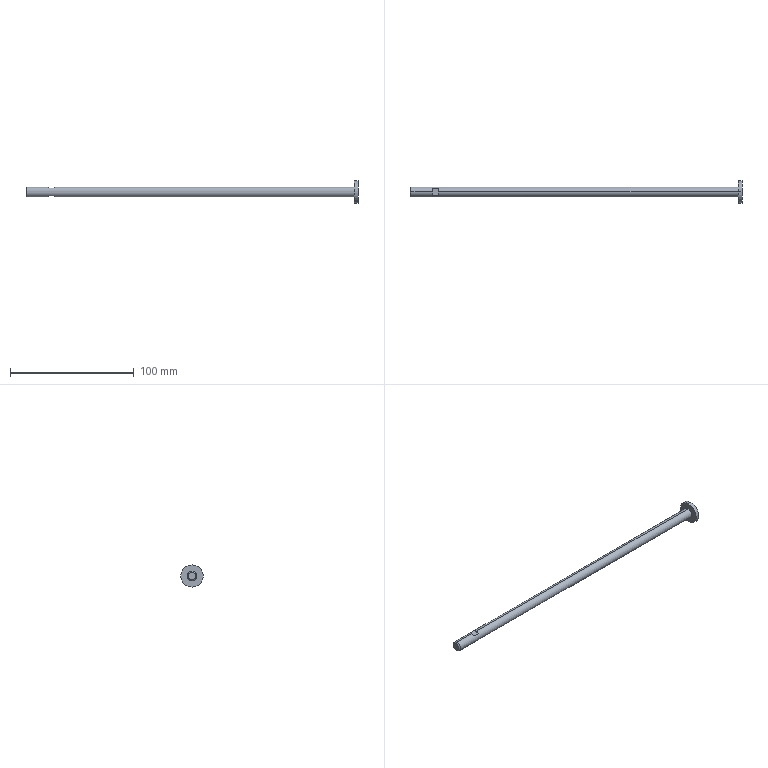Part | 1 solid | 15 faces | box 268 x 18 x 18 mm | volume 14041 mm3 | plane 9 | cylinder 4 | cone 2 | commonest cylinder face diameters 8 x2 18 x2
STEP:
#1=CARTESIAN_POINT('',(265.,0.,-9.));
#2=VERTEX_POINT('',#1);
#3=CARTESIAN_POINT('',(265.,0.,9.));
#4=VERTEX_POINT('',#3);
#5=CARTESIAN_POINT('',(265.,0.,0.));
#6=DIRECTION('',(1.,0.,0.));
#7=DIRECTION('',(0.,0.,-1.));
#8=AXIS2_PLACEMENT_3D('',#5,#6,#7);
#9=CIRCLE('',#8,9.);
#10=EDGE_CURVE('',#2,#4,#9,.T.);
#11=ORIENTED_EDGE('',*,*,#10,.T.);
#12=CARTESIAN_POINT('',(268.,0.,9.));
#13=VERTEX_POINT('',#12);
#14=CARTESIAN_POINT('',(268.,0.,9.));
#15=DIRECTION('',(1.,0.,0.));
#16=VECTOR('',#15,1000.);
#17=LINE('',#14,#16);
#18=EDGE_CURVE('',#4,#13,#17,.T.);
#19=ORIENTED_EDGE('',*,*,#18,.T.);
#20=CARTESIAN_POINT('',(268.,0.,-9.));
#21=VERTEX_POINT('',#20);
#22=CARTESIAN_POINT('',(268.,0.,0.));
#23=DIRECTION('',(1.,0.,0.));
#24=DIRECTION('',(0.,0.,-1.));
#25=AXIS2_PLACEMENT_3D('',#22,#23,#24);
#26=CIRCLE('',#25,9.);
#27=EDGE_CURVE('',#21,#13,#26,.T.);
#28=ORIENTED_EDGE('',*,*,#27,.F.);
#29=CARTESIAN_POINT('',(268.,0.,-9.));
#30=DIRECTION('',(1.,0.,0.));
#31=VECTOR('',#30,1000.);
#32=LINE('',#29,#31);
#33=EDGE_CURVE('',#2,#21,#32,.T.);
#34=ORIENTED_EDGE('',*,*,#33,.F.);
#35=EDGE_LOOP('',(#11,#19,#28,#34));
#36=FACE_OUTER_BOUND('',#35,.T.);
#37=CARTESIAN_POINT('',(268.,0.,0.));
#38=DIRECTION('',(1.,0.,0.));
#39=DIRECTION('',(0.,0.,-1.));
#40=AXIS2_PLACEMENT_3D('',#37,#38,#39);
#41=CYLINDRICAL_SURFACE('',#40,9.);
#42=ADVANCED_FACE('',(#36),#41,.T.);
#43=CARTESIAN_POINT('',(0.767,0.,-4.));
#44=VERTEX_POINT('',#43);
#45=CARTESIAN_POINT('',(0.767,0.,4.));
#46=VERTEX_POINT('',#45);
#47=CARTESIAN_POINT('',(0.767,0.,0.));
#48=DIRECTION('',(1.,0.,0.));
#49=DIRECTION('',(0.,0.,-1.));
#50=AXIS2_PLACEMENT_3D('',#47,#48,#49);
#51=CIRCLE('',#50,4.);
#52=EDGE_CURVE('',#44,#46,#51,.T.);
#53=ORIENTED_EDGE('',*,*,#52,.T.);
#54=CARTESIAN_POINT('',(18.,0.,4.));
#55=VERTEX_POINT('',#54);
#56=CARTESIAN_POINT('',(268.,0.,4.));
#57=DIRECTION('',(1.,0.,0.));
#58=VECTOR('',#57,1000.);
#59=LINE('',#56,#58);
#60=EDGE_CURVE('',#46,#55,#59,.T.);
#61=ORIENTED_EDGE('',*,*,#60,.T.);
#62=CARTESIAN_POINT('',(18.,2.646,3.));
#63=VERTEX_POINT('',#62);
#64=CARTESIAN_POINT('',(18.,0.,0.));
#65=DIRECTION('',(1.,0.,0.));
#66=DIRECTION('',(0.,0.,-1.));
#67=AXIS2_PLACEMENT_3D('',#64,#65,#66);
#68=CIRCLE('',#67,4.);
#69=EDGE_CURVE('',#63,#55,#68,.T.);
#70=ORIENTED_EDGE('',*,*,#69,.F.);
#71=CARTESIAN_POINT('',(23.,2.646,3.));
#72=VERTEX_POINT('',#71);
#73=CARTESIAN_POINT('',(268.,2.646,3.));
#74=DIRECTION('',(1.,0.,0.));
#75=VECTOR('',#74,1000.);
#76=LINE('',#73,#75);
#77=EDGE_CURVE('',#63,#72,#76,.T.);
#78=ORIENTED_EDGE('',*,*,#77,.T.);
#79=CARTESIAN_POINT('',(23.,0.,4.));
#80=VERTEX_POINT('',#79);
#81=CARTESIAN_POINT('',(23.,0.,0.));
#82=DIRECTION('',(1.,0.,0.));
#83=DIRECTION('',(0.,0.,-1.));
#84=AXIS2_PLACEMENT_3D('',#81,#82,#83);
#85=CIRCLE('',#84,4.);
#86=EDGE_CURVE('',#72,#80,#85,.T.);
#87=ORIENTED_EDGE('',*,*,#86,.T.);
#88=CARTESIAN_POINT('',(265.,0.,4.));
#89=VERTEX_POINT('',#88);
#90=CARTESIAN_POINT('',(268.,0.,4.));
#91=DIRECTION('',(1.,0.,0.));
#92=VECTOR('',#91,1000.);
#93=LINE('',#90,#92);
#94=EDGE_CURVE('',#80,#89,#93,.T.);
#95=ORIENTED_EDGE('',*,*,#94,.T.);
#96=CARTESIAN_POINT('',(265.,0.,-4.));
#97=VERTEX_POINT('',#96);
#98=CARTESIAN_POINT('',(265.,0.,0.));
#99=DIRECTION('',(1.,0.,0.));
#100=DIRECTION('',(0.,0.,-1.));
#101=AXIS2_PLACEMENT_3D('',#98,#99,#100);
#102=CIRCLE('',#101,4.);
#103=EDGE_CURVE('',#97,#89,#102,.T.);
#104=ORIENTED_EDGE('',*,*,#103,.F.);
#105=CARTESIAN_POINT('',(23.,0.,-4.));
#106=VERTEX_POINT('',#105);
#107=CARTESIAN_POINT('',(268.,0.,-4.));
#108=DIRECTION('',(1.,0.,0.));
#109=VECTOR('',#108,1000.);
#110=LINE('',#107,#109);
#111=EDGE_CURVE('',#106,#97,#110,.T.);
#112=ORIENTED_EDGE('',*,*,#111,.F.);
#113=CARTESIAN_POINT('',(23.,2.646,-3.));
#114=VERTEX_POINT('',#113);
#115=CARTESIAN_POINT('',(23.,0.,0.));
#116=DIRECTION('',(1.,0.,0.));
#117=DIRECTION('',(0.,0.,-1.));
#118=AXIS2_PLACEMENT_3D('',#115,#116,#117);
#119=CIRCLE('',#118,4.);
#120=EDGE_CURVE('',#106,#114,#119,.T.);
#121=ORIENTED_EDGE('',*,*,#120,.T.);
#122=CARTESIAN_POINT('',(18.,2.646,-3.));
#123=VERTEX_POINT('',#122);
#124=CARTESIAN_POINT('',(268.,2.646,-3.));
#125=DIRECTION('',(-1.,0.,0.));
#126=VECTOR('',#125,1000.);
#127=LINE('',#124,#126);
#128=EDGE_CURVE('',#114,#123,#127,.T.);
#129=ORIENTED_EDGE('',*,*,#128,.T.);
#130=CARTESIAN_POINT('',(18.,0.,-4.));
#131=VERTEX_POINT('',#130);
#132=CARTESIAN_POINT('',(18.,0.,0.));
#133=DIRECTION('',(1.,0.,0.));
#134=DIRECTION('',(0.,0.,-1.));
#135=AXIS2_PLACEMENT_3D('',#132,#133,#134);
#136=CIRCLE('',#135,4.);
#137=EDGE_CURVE('',#131,#123,#136,.T.);
#138=ORIENTED_EDGE('',*,*,#137,.F.);
#139=CARTESIAN_POINT('',(268.,0.,-4.));
#140=DIRECTION('',(1.,0.,0.));
#141=VECTOR('',#140,1000.);
#142=LINE('',#139,#141);
#143=EDGE_CURVE('',#44,#131,#142,.T.);
#144=ORIENTED_EDGE('',*,*,#143,.F.);
#145=EDGE_LOOP('',(#53,#61,#70,#78,#87,#95,#104,#112,#121,#129,#138,#144));
#146=FACE_OUTER_BOUND('',#145,.T.);
#147=CARTESIAN_POINT('',(268.,0.,0.));
#148=DIRECTION('',(1.,0.,0.));
#149=DIRECTION('',(0.,0.,-1.));
#150=AXIS2_PLACEMENT_3D('',#147,#148,#149);
#151=CYLINDRICAL_SURFACE('',#150,4.);
#152=ADVANCED_FACE('',(#146),#151,.T.);
#153=CARTESIAN_POINT('',(0.,0.,-3.233));
#154=VERTEX_POINT('',#153);
#155=CARTESIAN_POINT('',(0.,0.,3.233));
#156=VERTEX_POINT('',#155);
#157=CARTESIAN_POINT('',(0.,0.,0.));
#158=DIRECTION('',(1.,0.,0.));
#159=DIRECTION('',(0.,0.,-1.));
#160=AXIS2_PLACEMENT_3D('',#157,#158,#159);
#161=CIRCLE('',#160,3.233);
#162=EDGE_CURVE('',#154,#156,#161,.T.);
#163=ORIENTED_EDGE('',*,*,#162,.T.);
#164=CARTESIAN_POINT('',(0.,0.,3.233));
#165=DIRECTION('',(0.7071,0.,0.7071));
#166=VECTOR('',#165,1000.);
#167=LINE('',#164,#166);
#168=EDGE_CURVE('',#156,#46,#167,.T.);
#169=ORIENTED_EDGE('',*,*,#168,.T.);
#170=ORIENTED_EDGE('',*,*,#52,.F.);
#171=CARTESIAN_POINT('',(0.,0.,-3.233));
#172=DIRECTION('',(0.7071,0.,-0.7071));
#173=VECTOR('',#172,1000.);
#174=LINE('',#171,#173);
#175=EDGE_CURVE('',#154,#44,#174,.T.);
#176=ORIENTED_EDGE('',*,*,#175,.F.);
#177=EDGE_LOOP('',(#163,#169,#170,#176));
#178=FACE_OUTER_BOUND('',#177,.T.);
#179=CARTESIAN_POINT('',(0.,0.,0.));
#180=DIRECTION('',(1.,0.,0.));
#181=DIRECTION('',(0.,0.,-1.));
#182=AXIS2_PLACEMENT_3D('',#179,#180,#181);
#183=CONICAL_SURFACE('',#182,3.233,0.7854);
#184=ADVANCED_FACE('',(#178),#183,.T.);
#185=ORIENTED_EDGE('',*,*,#162,.F.);
#186=CARTESIAN_POINT('',(0.,0.,0.));
#187=DIRECTION('',(1.,0.,0.));
#188=DIRECTION('',(0.,0.,-1.));
#189=AXIS2_PLACEMENT_3D('',#186,#187,#188);
#190=CIRCLE('',#189,3.233);
#191=EDGE_CURVE('',#156,#154,#190,.T.);
#192=ORIENTED_EDGE('',*,*,#191,.F.);
#193=EDGE_LOOP('',(#185,#192));
#194=FACE_OUTER_BOUND('',#193,.T.);
#195=CARTESIAN_POINT('',(0.,0.,0.));
#196=DIRECTION('',(1.,0.,0.));
#197=DIRECTION('',(0.,1.,0.));
#198=AXIS2_PLACEMENT_3D('',#195,#196,#197);
#199=PLANE('',#198);
#200=ADVANCED_FACE('',(#194),#199,.F.);
#201=ORIENTED_EDGE('',*,*,#168,.F.);
#202=ORIENTED_EDGE('',*,*,#191,.T.);
#203=ORIENTED_EDGE('',*,*,#175,.T.);
#204=CARTESIAN_POINT('',(0.767,0.,0.));
#205=DIRECTION('',(1.,0.,0.));
#206=DIRECTION('',(0.,0.,-1.));
#207=AXIS2_PLACEMENT_3D('',#204,#205,#206);
#208=CIRCLE('',#207,4.);
#209=EDGE_CURVE('',#46,#44,#208,.T.);
#210=ORIENTED_EDGE('',*,*,#209,.F.);
#211=EDGE_LOOP('',(#201,#202,#203,#210));
#212=FACE_OUTER_BOUND('',#211,.T.);
#213=CARTESIAN_POINT('',(0.,0.,0.));
#214=DIRECTION('',(1.,0.,0.));
#215=DIRECTION('',(0.,0.,-1.));
#216=AXIS2_PLACEMENT_3D('',#213,#214,#215);
#217=CONICAL_SURFACE('',#216,3.233,0.7854);
#218=ADVANCED_FACE('',(#212),#217,.T.);
#219=ORIENTED_EDGE('',*,*,#60,.F.);
#220=ORIENTED_EDGE('',*,*,#209,.T.);
#221=ORIENTED_EDGE('',*,*,#143,.T.);
#222=CARTESIAN_POINT('',(18.,-2.646,-3.));
#223=VERTEX_POINT('',#222);
#224=CARTESIAN_POINT('',(18.,0.,0.));
#225=DIRECTION('',(1.,0.,0.));
#226=DIRECTION('',(0.,0.,-1.));
#227=AXIS2_PLACEMENT_3D('',#224,#225,#226);
#228=CIRCLE('',#227,4.);
#229=EDGE_CURVE('',#223,#131,#228,.T.);
#230=ORIENTED_EDGE('',*,*,#229,.F.);
#231=CARTESIAN_POINT('',(23.,-2.646,-3.));
#232=VERTEX_POINT('',#231);
#233=CARTESIAN_POINT('',(268.,-2.646,-3.));
#234=DIRECTION('',(1.,0.,0.));
#235=VECTOR('',#234,1000.);
#236=LINE('',#233,#235);
#237=EDGE_CURVE('',#223,#232,#236,.T.);
#238=ORIENTED_EDGE('',*,*,#237,.T.);
#239=CARTESIAN_POINT('',(23.,0.,0.));
#240=DIRECTION('',(1.,0.,0.));
#241=DIRECTION('',(0.,0.,-1.));
#242=AXIS2_PLACEMENT_3D('',#239,#240,#241);
#243=CIRCLE('',#242,4.);
#244=EDGE_CURVE('',#232,#106,#243,.T.);
#245=ORIENTED_EDGE('',*,*,#244,.T.);
#246=ORIENTED_EDGE('',*,*,#111,.T.);
#247=CARTESIAN_POINT('',(265.,0.,0.));
#248=DIRECTION('',(1.,0.,0.));
#249=DIRECTION('',(0.,0.,-1.));
#250=AXIS2_PLACEMENT_3D('',#247,#248,#249);
#251=CIRCLE('',#250,4.);
#252=EDGE_CURVE('',#89,#97,#251,.T.);
#253=ORIENTED_EDGE('',*,*,#252,.F.);
#254=ORIENTED_EDGE('',*,*,#94,.F.);
#255=CARTESIAN_POINT('',(23.,-2.646,3.));
#256=VERTEX_POINT('',#255);
#257=CARTESIAN_POINT('',(23.,0.,0.));
#258=DIRECTION('',(1.,0.,0.));
#259=DIRECTION('',(0.,0.,-1.));
#260=AXIS2_PLACEMENT_3D('',#257,#258,#259);
#261=CIRCLE('',#260,4.);
#262=EDGE_CURVE('',#80,#256,#261,.T.);
#263=ORIENTED_EDGE('',*,*,#262,.T.);
#264=CARTESIAN_POINT('',(18.,-2.646,3.));
#265=VERTEX_POINT('',#264);
#266=CARTESIAN_POINT('',(268.,-2.646,3.));
#267=DIRECTION('',(-1.,0.,0.));
#268=VECTOR('',#267,1000.);
#269=LINE('',#266,#268);
#270=EDGE_CURVE('',#256,#265,#269,.T.);
#271=ORIENTED_EDGE('',*,*,#270,.T.);
#272=CARTESIAN_POINT('',(18.,0.,0.));
#273=DIRECTION('',(1.,0.,0.));
#274=DIRECTION('',(0.,0.,-1.));
#275=AXIS2_PLACEMENT_3D('',#272,#273,#274);
#276=CIRCLE('',#275,4.);
#277=EDGE_CURVE('',#55,#265,#276,.T.);
#278=ORIENTED_EDGE('',*,*,#277,.F.);
#279=EDGE_LOOP('',(#219,#220,#221,#230,#238,#245,#246,#253,#254,#263,#271,#278));
#280=FACE_OUTER_BOUND('',#279,.T.);
#281=CARTESIAN_POINT('',(268.,0.,0.));
#282=DIRECTION('',(1.,0.,0.));
#283=DIRECTION('',(0.,0.,-1.));
#284=AXIS2_PLACEMENT_3D('',#281,#282,#283);
#285=CYLINDRICAL_SURFACE('',#284,4.);
#286=ADVANCED_FACE('',(#280),#285,.T.);
#287=ORIENTED_EDGE('',*,*,#10,.F.);
#288=CARTESIAN_POINT('',(265.,0.,0.));
#289=DIRECTION('',(1.,0.,0.));
#290=DIRECTION('',(0.,0.,-1.));
#291=AXIS2_PLACEMENT_3D('',#288,#289,#290);
#292=CIRCLE('',#291,9.);
#293=EDGE_CURVE('',#4,#2,#292,.T.);
#294=ORIENTED_EDGE('',*,*,#293,.F.);
#295=EDGE_LOOP('',(#287,#294));
#296=FACE_OUTER_BOUND('',#295,.T.);
#297=ORIENTED_EDGE('',*,*,#103,.T.);
#298=ORIENTED_EDGE('',*,*,#252,.T.);
#299=EDGE_LOOP('',(#297,#298));
#300=FACE_BOUND('',#299,.T.);
#301=CARTESIAN_POINT('',(265.,4.,0.));
#302=DIRECTION('',(1.,0.,0.));
#303=DIRECTION('',(0.,1.,0.));
#304=AXIS2_PLACEMENT_3D('',#301,#302,#303);
#305=PLANE('',#304);
#306=ADVANCED_FACE('',(#296,#300),#305,.F.);
#307=ORIENTED_EDGE('',*,*,#18,.F.);
#308=ORIENTED_EDGE('',*,*,#293,.T.);
#309=ORIENTED_EDGE('',*,*,#33,.T.);
#310=CARTESIAN_POINT('',(268.,0.,0.));
#311=DIRECTION('',(1.,0.,0.));
#312=DIRECTION('',(0.,0.,-1.));
#313=AXIS2_PLACEMENT_3D('',#310,#311,#312);
#314=CIRCLE('',#313,9.);
#315=EDGE_CURVE('',#13,#21,#314,.T.);
#316=ORIENTED_EDGE('',*,*,#315,.F.);
#317=EDGE_LOOP('',(#307,#308,#309,#316));
#318=FACE_OUTER_BOUND('',#317,.T.);
#319=CARTESIAN_POINT('',(268.,0.,0.));
#320=DIRECTION('',(1.,0.,0.));
#321=DIRECTION('',(0.,0.,-1.));
#322=AXIS2_PLACEMENT_3D('',#319,#320,#321);
#323=CYLINDRICAL_SURFACE('',#322,9.);
#324=ADVANCED_FACE('',(#318),#323,.T.);
#325=ORIENTED_EDGE('',*,*,#27,.T.);
#326=ORIENTED_EDGE('',*,*,#315,.T.);
#327=EDGE_LOOP('',(#325,#326));
#328=FACE_OUTER_BOUND('',#327,.T.);
#329=CARTESIAN_POINT('',(268.,9.,0.));
#330=DIRECTION('',(-1.,0.,0.));
#331=DIRECTION('',(0.,0.,1.));
#332=AXIS2_PLACEMENT_3D('',#329,#330,#331);
#333=PLANE('',#332);
#334=ADVANCED_FACE('',(#328),#333,.F.);
#335=CARTESIAN_POINT('',(23.,-50.,-3.));
#336=DIRECTION('',(0.,1.,0.));
#337=VECTOR('',#336,1000.);
#338=LINE('',#335,#337);
#339=EDGE_CURVE('',#232,#114,#338,.T.);
#340=ORIENTED_EDGE('',*,*,#339,.T.);
#341=ORIENTED_EDGE('',*,*,#120,.F.);
#342=ORIENTED_EDGE('',*,*,#244,.F.);
#343=EDGE_LOOP('',(#340,#341,#342));
#344=FACE_OUTER_BOUND('',#343,.T.);
#345=CARTESIAN_POINT('',(23.,0.,0.));
#346=DIRECTION('',(1.,0.,0.));
#347=DIRECTION('',(0.,1.,0.));
#348=AXIS2_PLACEMENT_3D('',#345,#346,#347);
#349=PLANE('',#348);
#350=ADVANCED_FACE('',(#344),#349,.F.);
#351=ORIENTED_EDGE('',*,*,#229,.T.);
#352=ORIENTED_EDGE('',*,*,#137,.T.);
#353=CARTESIAN_POINT('',(18.,-50.,-3.));
#354=DIRECTION('',(0.,1.,0.));
#355=VECTOR('',#354,1000.);
#356=LINE('',#353,#355);
#357=EDGE_CURVE('',#223,#123,#356,.T.);
#358=ORIENTED_EDGE('',*,*,#357,.F.);
#359=EDGE_LOOP('',(#351,#352,#358));
#360=FACE_OUTER_BOUND('',#359,.T.);
#361=CARTESIAN_POINT('',(18.,0.,0.));
#362=DIRECTION('',(1.,0.,0.));
#363=DIRECTION('',(0.,1.,0.));
#364=AXIS2_PLACEMENT_3D('',#361,#362,#363);
#365=PLANE('',#364);
#366=ADVANCED_FACE('',(#360),#365,.T.);
#367=ORIENTED_EDGE('',*,*,#357,.T.);
#368=ORIENTED_EDGE('',*,*,#128,.F.);
#369=ORIENTED_EDGE('',*,*,#339,.F.);
#370=ORIENTED_EDGE('',*,*,#237,.F.);
#371=EDGE_LOOP('',(#367,#368,#369,#370));
#372=FACE_OUTER_BOUND('',#371,.T.);
#373=CARTESIAN_POINT('',(23.,-50.,-3.));
#374=DIRECTION('',(0.,0.,1.));
#375=DIRECTION('',(0.,-1.,0.));
#376=AXIS2_PLACEMENT_3D('',#373,#374,#375);
#377=PLANE('',#376);
#378=ADVANCED_FACE('',(#372),#377,.F.);
#379=CARTESIAN_POINT('',(18.,50.,3.));
#380=DIRECTION('',(0.,-1.,0.));
#381=VECTOR('',#380,1000.);
#382=LINE('',#379,#381);
#383=EDGE_CURVE('',#63,#265,#382,.T.);
#384=ORIENTED_EDGE('',*,*,#383,.T.);
#385=ORIENTED_EDGE('',*,*,#270,.F.);
#386=CARTESIAN_POINT('',(23.,50.,3.));
#387=DIRECTION('',(0.,-1.,0.));
#388=VECTOR('',#387,1000.);
#389=LINE('',#386,#388);
#390=EDGE_CURVE('',#72,#256,#389,.T.);
#391=ORIENTED_EDGE('',*,*,#390,.F.);
#392=ORIENTED_EDGE('',*,*,#77,.F.);
#393=EDGE_LOOP('',(#384,#385,#391,#392));
#394=FACE_OUTER_BOUND('',#393,.T.);
#395=CARTESIAN_POINT('',(23.,50.,3.));
#396=DIRECTION('',(0.,0.,-1.));
#397=DIRECTION('',(-1.,0.,0.));
#398=AXIS2_PLACEMENT_3D('',#395,#396,#397);
#399=PLANE('',#398);
#400=ADVANCED_FACE('',(#394),#399,.F.);
#401=ORIENTED_EDGE('',*,*,#390,.T.);
#402=ORIENTED_EDGE('',*,*,#262,.F.);
#403=ORIENTED_EDGE('',*,*,#86,.F.);
#404=EDGE_LOOP('',(#401,#402,#403));
#405=FACE_OUTER_BOUND('',#404,.T.);
#406=CARTESIAN_POINT('',(23.,0.,0.));
#407=DIRECTION('',(1.,0.,0.));
#408=DIRECTION('',(0.,1.,0.));
#409=AXIS2_PLACEMENT_3D('',#406,#407,#408);
#410=PLANE('',#409);
#411=ADVANCED_FACE('',(#405),#410,.F.);
#412=ORIENTED_EDGE('',*,*,#69,.T.);
#413=ORIENTED_EDGE('',*,*,#277,.T.);
#414=ORIENTED_EDGE('',*,*,#383,.F.);
#415=EDGE_LOOP('',(#412,#413,#414));
#416=FACE_OUTER_BOUND('',#415,.T.);
#417=CARTESIAN_POINT('',(18.,0.,0.));
#418=DIRECTION('',(1.,0.,0.));
#419=DIRECTION('',(0.,1.,0.));
#420=AXIS2_PLACEMENT_3D('',#417,#418,#419);
#421=PLANE('',#420);
#422=ADVANCED_FACE('',(#416),#421,.T.);
#423=CLOSED_SHELL('',(#42,#152,#184,#200,#218,#286,#306,#324,#334,#350,#366,#378,#400,#411,#422));
#424=MANIFOLD_SOLID_BREP('',#423);
#425=CARTESIAN_POINT('',(0.,0.,0.));
#426=DIRECTION('',(0.,0.,1.));
#427=DIRECTION('',(1.,0.,0.));
#428=AXIS2_PLACEMENT_3D('',#425,#426,#427);
#429=(LENGTH_UNIT()NAMED_UNIT(*)SI_UNIT(.MILLI.,.METRE.));
#430=UNCERTAINTY_MEASURE_WITH_UNIT(LENGTH_MEASURE(0.00001),#429,'','');
#431=(NAMED_UNIT(*)PLANE_ANGLE_UNIT()SI_UNIT($,.RADIAN.));
#432=(NAMED_UNIT(*)SI_UNIT($,.STERADIAN.)SOLID_ANGLE_UNIT());
#433=(GEOMETRIC_REPRESENTATION_CONTEXT(3)GLOBAL_UNCERTAINTY_ASSIGNED_CONTEXT((#430))GLOBAL_UNIT_ASSIGNED_CONTEXT((#429,#431,#432))REPRESENTATION_CONTEXT('',''));
#434=ADVANCED_BREP_SHAPE_REPRESENTATION('',(#424,#428),#433);